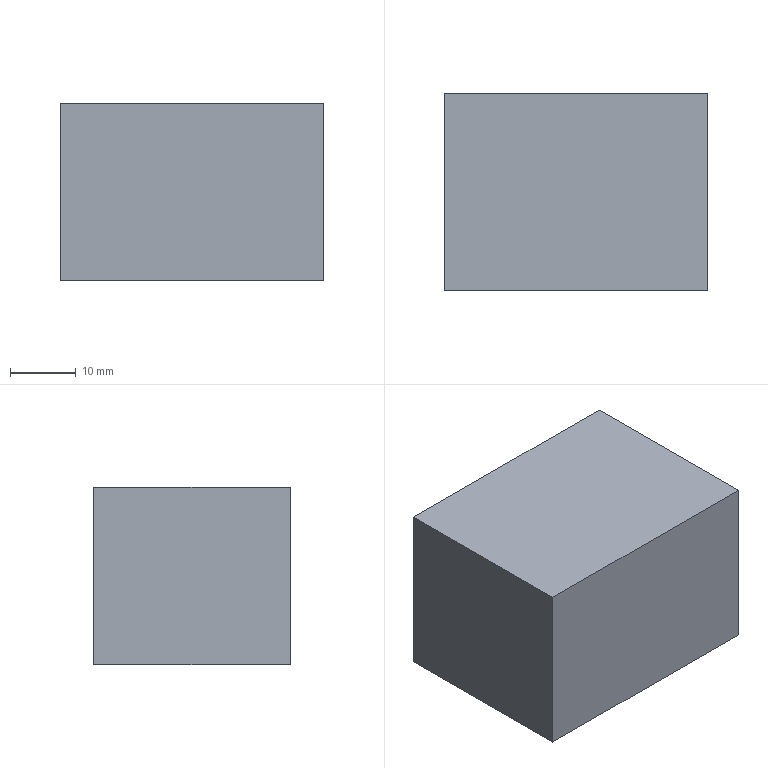Part | SolidWorks | features Extrusion 1 | 1 solid | 6 faces | box 40 x 30 x 27 mm | volume 32400 mm3 | plane 6
STEP:
#1=CARTESIAN_POINT('',(-20.,15.,0.));
#2=VERTEX_POINT('',#1);
#3=CARTESIAN_POINT('',(-20.,-15.,0.));
#4=VERTEX_POINT('',#3);
#5=CARTESIAN_POINT('',(-20.,15.,0.));
#6=DIRECTION('',(0.,-1.,0.));
#7=VECTOR('',#6,1000.);
#8=LINE('',#5,#7);
#9=EDGE_CURVE('',#2,#4,#8,.T.);
#10=ORIENTED_EDGE('',*,*,#9,.T.);
#11=CARTESIAN_POINT('',(-20.,-15.,27.));
#12=VERTEX_POINT('',#11);
#13=CARTESIAN_POINT('',(-20.,-15.,27.));
#14=DIRECTION('',(0.,0.,-1.));
#15=VECTOR('',#14,1000.);
#16=LINE('',#13,#15);
#17=EDGE_CURVE('',#12,#4,#16,.T.);
#18=ORIENTED_EDGE('',*,*,#17,.F.);
#19=CARTESIAN_POINT('',(-20.,15.,27.));
#20=VERTEX_POINT('',#19);
#21=CARTESIAN_POINT('',(-20.,15.,27.));
#22=DIRECTION('',(0.,-1.,0.));
#23=VECTOR('',#22,1000.);
#24=LINE('',#21,#23);
#25=EDGE_CURVE('',#20,#12,#24,.T.);
#26=ORIENTED_EDGE('',*,*,#25,.F.);
#27=CARTESIAN_POINT('',(-20.,15.,27.));
#28=DIRECTION('',(0.,0.,-1.));
#29=VECTOR('',#28,1000.);
#30=LINE('',#27,#29);
#31=EDGE_CURVE('',#20,#2,#30,.T.);
#32=ORIENTED_EDGE('',*,*,#31,.T.);
#33=EDGE_LOOP('',(#10,#18,#26,#32));
#34=FACE_OUTER_BOUND('',#33,.T.);
#35=CARTESIAN_POINT('',(-20.,15.,27.));
#36=DIRECTION('',(1.,0.,0.));
#37=DIRECTION('',(0.,0.,-1.));
#38=AXIS2_PLACEMENT_3D('',#35,#36,#37);
#39=PLANE('',#38);
#40=ADVANCED_FACE('',(#34),#39,.F.);
#41=CARTESIAN_POINT('',(20.,-15.,0.));
#42=VERTEX_POINT('',#41);
#43=CARTESIAN_POINT('',(20.,-15.,0.));
#44=DIRECTION('',(1.,0.,0.));
#45=VECTOR('',#44,1000.);
#46=LINE('',#43,#45);
#47=EDGE_CURVE('',#4,#42,#46,.T.);
#48=ORIENTED_EDGE('',*,*,#47,.T.);
#49=CARTESIAN_POINT('',(20.,-15.,27.));
#50=VERTEX_POINT('',#49);
#51=CARTESIAN_POINT('',(20.,-15.,27.));
#52=DIRECTION('',(0.,0.,-1.));
#53=VECTOR('',#52,1000.);
#54=LINE('',#51,#53);
#55=EDGE_CURVE('',#50,#42,#54,.T.);
#56=ORIENTED_EDGE('',*,*,#55,.F.);
#57=CARTESIAN_POINT('',(20.,-15.,27.));
#58=DIRECTION('',(1.,0.,0.));
#59=VECTOR('',#58,1000.);
#60=LINE('',#57,#59);
#61=EDGE_CURVE('',#12,#50,#60,.T.);
#62=ORIENTED_EDGE('',*,*,#61,.F.);
#63=ORIENTED_EDGE('',*,*,#17,.T.);
#64=EDGE_LOOP('',(#48,#56,#62,#63));
#65=FACE_OUTER_BOUND('',#64,.T.);
#66=CARTESIAN_POINT('',(20.,-15.,27.));
#67=DIRECTION('',(0.,1.,0.));
#68=DIRECTION('',(-1.,0.,0.));
#69=AXIS2_PLACEMENT_3D('',#66,#67,#68);
#70=PLANE('',#69);
#71=ADVANCED_FACE('',(#65),#70,.F.);
#72=CARTESIAN_POINT('',(20.,15.,0.));
#73=VERTEX_POINT('',#72);
#74=CARTESIAN_POINT('',(20.,15.,0.));
#75=DIRECTION('',(0.,1.,0.));
#76=VECTOR('',#75,1000.);
#77=LINE('',#74,#76);
#78=EDGE_CURVE('',#42,#73,#77,.T.);
#79=ORIENTED_EDGE('',*,*,#78,.T.);
#80=CARTESIAN_POINT('',(20.,15.,27.));
#81=VERTEX_POINT('',#80);
#82=CARTESIAN_POINT('',(20.,15.,27.));
#83=DIRECTION('',(0.,0.,-1.));
#84=VECTOR('',#83,1000.);
#85=LINE('',#82,#84);
#86=EDGE_CURVE('',#81,#73,#85,.T.);
#87=ORIENTED_EDGE('',*,*,#86,.F.);
#88=CARTESIAN_POINT('',(20.,15.,27.));
#89=DIRECTION('',(0.,1.,0.));
#90=VECTOR('',#89,1000.);
#91=LINE('',#88,#90);
#92=EDGE_CURVE('',#50,#81,#91,.T.);
#93=ORIENTED_EDGE('',*,*,#92,.F.);
#94=ORIENTED_EDGE('',*,*,#55,.T.);
#95=EDGE_LOOP('',(#79,#87,#93,#94));
#96=FACE_OUTER_BOUND('',#95,.T.);
#97=CARTESIAN_POINT('',(20.,15.,27.));
#98=DIRECTION('',(-1.,0.,0.));
#99=DIRECTION('',(0.,-1.,0.));
#100=AXIS2_PLACEMENT_3D('',#97,#98,#99);
#101=PLANE('',#100);
#102=ADVANCED_FACE('',(#96),#101,.F.);
#103=CARTESIAN_POINT('',(20.,15.,0.));
#104=DIRECTION('',(-1.,0.,0.));
#105=VECTOR('',#104,1000.);
#106=LINE('',#103,#105);
#107=EDGE_CURVE('',#73,#2,#106,.T.);
#108=ORIENTED_EDGE('',*,*,#107,.T.);
#109=ORIENTED_EDGE('',*,*,#31,.F.);
#110=CARTESIAN_POINT('',(20.,15.,27.));
#111=DIRECTION('',(-1.,0.,0.));
#112=VECTOR('',#111,1000.);
#113=LINE('',#110,#112);
#114=EDGE_CURVE('',#81,#20,#113,.T.);
#115=ORIENTED_EDGE('',*,*,#114,.F.);
#116=ORIENTED_EDGE('',*,*,#86,.T.);
#117=EDGE_LOOP('',(#108,#109,#115,#116));
#118=FACE_OUTER_BOUND('',#117,.T.);
#119=CARTESIAN_POINT('',(20.,15.,27.));
#120=DIRECTION('',(0.,-1.,0.));
#121=DIRECTION('',(1.,0.,0.));
#122=AXIS2_PLACEMENT_3D('',#119,#120,#121);
#123=PLANE('',#122);
#124=ADVANCED_FACE('',(#118),#123,.F.);
#125=ORIENTED_EDGE('',*,*,#25,.T.);
#126=ORIENTED_EDGE('',*,*,#61,.T.);
#127=ORIENTED_EDGE('',*,*,#92,.T.);
#128=ORIENTED_EDGE('',*,*,#114,.T.);
#129=EDGE_LOOP('',(#125,#126,#127,#128));
#130=FACE_OUTER_BOUND('',#129,.T.);
#131=CARTESIAN_POINT('',(0.,0.,27.));
#132=DIRECTION('',(0.,0.,-1.));
#133=DIRECTION('',(-1.,0.,0.));
#134=AXIS2_PLACEMENT_3D('',#131,#132,#133);
#135=PLANE('',#134);
#136=ADVANCED_FACE('',(#130),#135,.F.);
#137=ORIENTED_EDGE('',*,*,#9,.F.);
#138=ORIENTED_EDGE('',*,*,#107,.F.);
#139=ORIENTED_EDGE('',*,*,#78,.F.);
#140=ORIENTED_EDGE('',*,*,#47,.F.);
#141=EDGE_LOOP('',(#137,#138,#139,#140));
#142=FACE_OUTER_BOUND('',#141,.T.);
#143=CARTESIAN_POINT('',(0.,0.,0.));
#144=DIRECTION('',(0.,0.,-1.));
#145=DIRECTION('',(-1.,0.,0.));
#146=AXIS2_PLACEMENT_3D('',#143,#144,#145);
#147=PLANE('',#146);
#148=ADVANCED_FACE('',(#142),#147,.T.);
#149=CLOSED_SHELL('',(#40,#71,#102,#124,#136,#148));
#150=MANIFOLD_SOLID_BREP('',#149);
#151=CARTESIAN_POINT('',(0.,0.,0.));
#152=DIRECTION('',(0.,0.,1.));
#153=DIRECTION('',(1.,0.,0.));
#154=AXIS2_PLACEMENT_3D('',#151,#152,#153);
#155=(LENGTH_UNIT()NAMED_UNIT(*)SI_UNIT(.MILLI.,.METRE.));
#156=UNCERTAINTY_MEASURE_WITH_UNIT(LENGTH_MEASURE(0.00001),#155,'','');
#157=(NAMED_UNIT(*)PLANE_ANGLE_UNIT()SI_UNIT($,.RADIAN.));
#158=(NAMED_UNIT(*)SI_UNIT($,.STERADIAN.)SOLID_ANGLE_UNIT());
#159=(GEOMETRIC_REPRESENTATION_CONTEXT(3)GLOBAL_UNCERTAINTY_ASSIGNED_CONTEXT((#156))GLOBAL_UNIT_ASSIGNED_CONTEXT((#155,#157,#158))REPRESENTATION_CONTEXT('',''));
#160=ADVANCED_BREP_SHAPE_REPRESENTATION('',(#150,#154),#159);